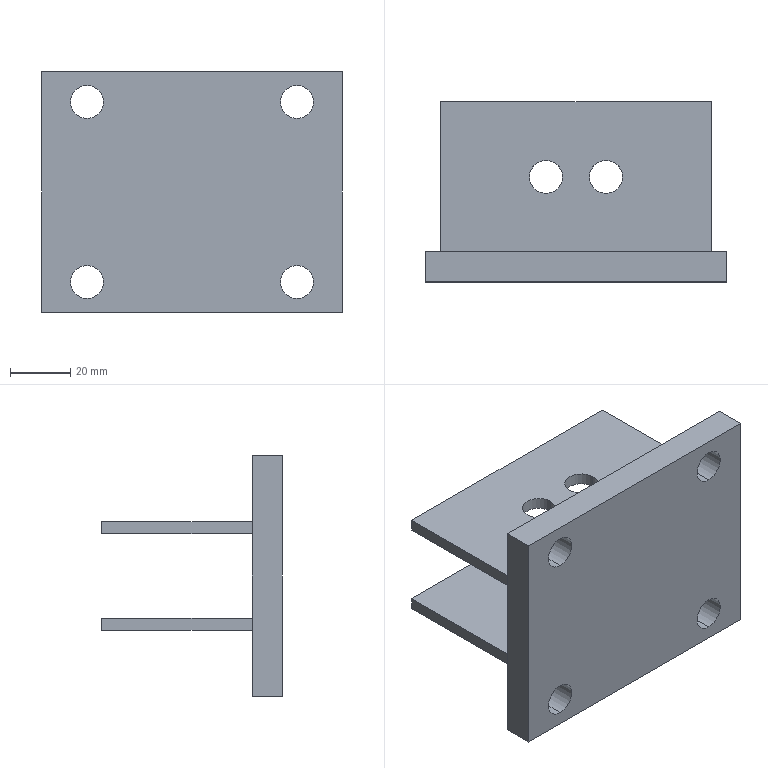Part | SolidWorks | features ICE 3, Extrusion 1, MirrorPattern 1 | 1 solid | 32 faces | box 100 x 60 x 80 mm | volume 110678 mm3 | cylinder 16 | plane 16 | commonest cylinder face diameters 11 x16
STEP:
#1=CARTESIAN_POINT('',(4.5,0.,-32.));
#2=VERTEX_POINT('',#1);
#3=CARTESIAN_POINT('',(15.5,0.,-32.));
#4=VERTEX_POINT('',#3);
#5=CARTESIAN_POINT('',(10.,0.,-32.));
#6=DIRECTION('',(0.,0.,1.));
#7=DIRECTION('',(1.,0.,0.));
#8=AXIS2_PLACEMENT_3D('',#5,#6,#7);
#9=CIRCLE('',#8,5.5);
#10=EDGE_CURVE('',#2,#4,#9,.T.);
#11=ORIENTED_EDGE('',*,*,#10,.F.);
#12=CARTESIAN_POINT('',(4.5,0.,-28.));
#13=VERTEX_POINT('',#12);
#14=CARTESIAN_POINT('',(4.5,0.,-54.));
#15=DIRECTION('',(0.,0.,1.));
#16=VECTOR('',#15,1000.);
#17=LINE('',#14,#16);
#18=EDGE_CURVE('',#2,#13,#17,.T.);
#19=ORIENTED_EDGE('',*,*,#18,.T.);
#20=CARTESIAN_POINT('',(15.5,0.,-28.));
#21=VERTEX_POINT('',#20);
#22=CARTESIAN_POINT('',(10.,0.,-28.));
#23=DIRECTION('',(0.,0.,1.));
#24=DIRECTION('',(1.,0.,0.));
#25=AXIS2_PLACEMENT_3D('',#22,#23,#24);
#26=CIRCLE('',#25,5.5);
#27=EDGE_CURVE('',#13,#21,#26,.T.);
#28=ORIENTED_EDGE('',*,*,#27,.T.);
#29=CARTESIAN_POINT('',(15.5,0.,-54.));
#30=DIRECTION('',(0.,0.,1.));
#31=VECTOR('',#30,1000.);
#32=LINE('',#29,#31);
#33=EDGE_CURVE('',#4,#21,#32,.T.);
#34=ORIENTED_EDGE('',*,*,#33,.F.);
#35=EDGE_LOOP('',(#11,#19,#28,#34));
#36=FACE_OUTER_BOUND('',#35,.T.);
#37=CARTESIAN_POINT('',(10.,0.,-54.));
#38=DIRECTION('',(0.,0.,1.));
#39=DIRECTION('',(1.,0.,0.));
#40=AXIS2_PLACEMENT_3D('',#37,#38,#39);
#41=CYLINDRICAL_SURFACE('',#40,5.5);
#42=ADVANCED_FACE('',(#36),#41,.F.);
#43=CARTESIAN_POINT('',(-15.5,0.,-32.));
#44=VERTEX_POINT('',#43);
#45=CARTESIAN_POINT('',(-4.5,0.,-32.));
#46=VERTEX_POINT('',#45);
#47=CARTESIAN_POINT('',(-10.,0.,-32.));
#48=DIRECTION('',(0.,0.,1.));
#49=DIRECTION('',(1.,0.,0.));
#50=AXIS2_PLACEMENT_3D('',#47,#48,#49);
#51=CIRCLE('',#50,5.5);
#52=EDGE_CURVE('',#44,#46,#51,.T.);
#53=ORIENTED_EDGE('',*,*,#52,.F.);
#54=CARTESIAN_POINT('',(-15.5,0.,-28.));
#55=VERTEX_POINT('',#54);
#56=CARTESIAN_POINT('',(-15.5,0.,-54.));
#57=DIRECTION('',(0.,0.,1.));
#58=VECTOR('',#57,1000.);
#59=LINE('',#56,#58);
#60=EDGE_CURVE('',#44,#55,#59,.T.);
#61=ORIENTED_EDGE('',*,*,#60,.T.);
#62=CARTESIAN_POINT('',(-4.5,0.,-28.));
#63=VERTEX_POINT('',#62);
#64=CARTESIAN_POINT('',(-10.,0.,-28.));
#65=DIRECTION('',(0.,0.,1.));
#66=DIRECTION('',(1.,0.,0.));
#67=AXIS2_PLACEMENT_3D('',#64,#65,#66);
#68=CIRCLE('',#67,5.5);
#69=EDGE_CURVE('',#55,#63,#68,.T.);
#70=ORIENTED_EDGE('',*,*,#69,.T.);
#71=CARTESIAN_POINT('',(-4.5,0.,-54.));
#72=DIRECTION('',(0.,0.,1.));
#73=VECTOR('',#72,1000.);
#74=LINE('',#71,#73);
#75=EDGE_CURVE('',#46,#63,#74,.T.);
#76=ORIENTED_EDGE('',*,*,#75,.F.);
#77=EDGE_LOOP('',(#53,#61,#70,#76));
#78=FACE_OUTER_BOUND('',#77,.T.);
#79=CARTESIAN_POINT('',(-10.,0.,-54.));
#80=DIRECTION('',(0.,0.,1.));
#81=DIRECTION('',(1.,0.,0.));
#82=AXIS2_PLACEMENT_3D('',#79,#80,#81);
#83=CYLINDRICAL_SURFACE('',#82,5.5);
#84=ADVANCED_FACE('',(#78),#83,.F.);
#85=CARTESIAN_POINT('',(-35.,-35.,-38.5));
#86=VERTEX_POINT('',#85);
#87=CARTESIAN_POINT('',(-35.,-35.,-49.5));
#88=VERTEX_POINT('',#87);
#89=CARTESIAN_POINT('',(-35.,-35.,-44.));
#90=DIRECTION('',(0.,-1.,0.));
#91=DIRECTION('',(0.,0.,-1.));
#92=AXIS2_PLACEMENT_3D('',#89,#90,#91);
#93=CIRCLE('',#92,5.5);
#94=EDGE_CURVE('',#86,#88,#93,.T.);
#95=ORIENTED_EDGE('',*,*,#94,.T.);
#96=CARTESIAN_POINT('',(-35.,-25.,-49.5));
#97=VERTEX_POINT('',#96);
#98=CARTESIAN_POINT('',(-35.,-35.,-49.5));
#99=DIRECTION('',(0.,1.,0.));
#100=VECTOR('',#99,1000.);
#101=LINE('',#98,#100);
#102=EDGE_CURVE('',#88,#97,#101,.T.);
#103=ORIENTED_EDGE('',*,*,#102,.T.);
#104=CARTESIAN_POINT('',(-35.,-25.,-38.5));
#105=VERTEX_POINT('',#104);
#106=CARTESIAN_POINT('',(-35.,-25.,-44.));
#107=DIRECTION('',(0.,-1.,0.));
#108=DIRECTION('',(0.,0.,-1.));
#109=AXIS2_PLACEMENT_3D('',#106,#107,#108);
#110=CIRCLE('',#109,5.5);
#111=EDGE_CURVE('',#105,#97,#110,.T.);
#112=ORIENTED_EDGE('',*,*,#111,.F.);
#113=CARTESIAN_POINT('',(-35.,-35.,-38.5));
#114=DIRECTION('',(0.,1.,0.));
#115=VECTOR('',#114,1000.);
#116=LINE('',#113,#115);
#117=EDGE_CURVE('',#86,#105,#116,.T.);
#118=ORIENTED_EDGE('',*,*,#117,.F.);
#119=EDGE_LOOP('',(#95,#103,#112,#118));
#120=FACE_OUTER_BOUND('',#119,.T.);
#121=CARTESIAN_POINT('',(-35.,-35.,-44.));
#122=DIRECTION('',(0.,1.,0.));
#123=DIRECTION('',(0.,0.,1.));
#124=AXIS2_PLACEMENT_3D('',#121,#122,#123);
#125=CYLINDRICAL_SURFACE('',#124,5.5);
#126=ADVANCED_FACE('',(#120),#125,.F.);
#127=CARTESIAN_POINT('',(35.,-35.,-38.5));
#128=VERTEX_POINT('',#127);
#129=CARTESIAN_POINT('',(35.,-35.,-49.5));
#130=VERTEX_POINT('',#129);
#131=CARTESIAN_POINT('',(35.,-35.,-44.));
#132=DIRECTION('',(0.,-1.,0.));
#133=DIRECTION('',(0.,0.,-1.));
#134=AXIS2_PLACEMENT_3D('',#131,#132,#133);
#135=CIRCLE('',#134,5.5);
#136=EDGE_CURVE('',#128,#130,#135,.T.);
#137=ORIENTED_EDGE('',*,*,#136,.T.);
#138=CARTESIAN_POINT('',(35.,-25.,-49.5));
#139=VERTEX_POINT('',#138);
#140=CARTESIAN_POINT('',(35.,-35.,-49.5));
#141=DIRECTION('',(0.,1.,0.));
#142=VECTOR('',#141,1000.);
#143=LINE('',#140,#142);
#144=EDGE_CURVE('',#130,#139,#143,.T.);
#145=ORIENTED_EDGE('',*,*,#144,.T.);
#146=CARTESIAN_POINT('',(35.,-25.,-38.5));
#147=VERTEX_POINT('',#146);
#148=CARTESIAN_POINT('',(35.,-25.,-44.));
#149=DIRECTION('',(0.,-1.,0.));
#150=DIRECTION('',(0.,0.,-1.));
#151=AXIS2_PLACEMENT_3D('',#148,#149,#150);
#152=CIRCLE('',#151,5.5);
#153=EDGE_CURVE('',#147,#139,#152,.T.);
#154=ORIENTED_EDGE('',*,*,#153,.F.);
#155=CARTESIAN_POINT('',(35.,-35.,-38.5));
#156=DIRECTION('',(0.,1.,0.));
#157=VECTOR('',#156,1000.);
#158=LINE('',#155,#157);
#159=EDGE_CURVE('',#128,#147,#158,.T.);
#160=ORIENTED_EDGE('',*,*,#159,.F.);
#161=EDGE_LOOP('',(#137,#145,#154,#160));
#162=FACE_OUTER_BOUND('',#161,.T.);
#163=CARTESIAN_POINT('',(35.,-35.,-44.));
#164=DIRECTION('',(0.,1.,0.));
#165=DIRECTION('',(0.,0.,1.));
#166=AXIS2_PLACEMENT_3D('',#163,#164,#165);
#167=CYLINDRICAL_SURFACE('',#166,5.5);
#168=ADVANCED_FACE('',(#162),#167,.F.);
#169=CARTESIAN_POINT('',(35.,-35.,21.5));
#170=VERTEX_POINT('',#169);
#171=CARTESIAN_POINT('',(35.,-35.,10.5));
#172=VERTEX_POINT('',#171);
#173=CARTESIAN_POINT('',(35.,-35.,16.));
#174=DIRECTION('',(0.,-1.,0.));
#175=DIRECTION('',(0.,0.,-1.));
#176=AXIS2_PLACEMENT_3D('',#173,#174,#175);
#177=CIRCLE('',#176,5.5);
#178=EDGE_CURVE('',#170,#172,#177,.T.);
#179=ORIENTED_EDGE('',*,*,#178,.T.);
#180=CARTESIAN_POINT('',(35.,-25.,10.5));
#181=VERTEX_POINT('',#180);
#182=CARTESIAN_POINT('',(35.,-35.,10.5));
#183=DIRECTION('',(0.,1.,0.));
#184=VECTOR('',#183,1000.);
#185=LINE('',#182,#184);
#186=EDGE_CURVE('',#172,#181,#185,.T.);
#187=ORIENTED_EDGE('',*,*,#186,.T.);
#188=CARTESIAN_POINT('',(35.,-25.,21.5));
#189=VERTEX_POINT('',#188);
#190=CARTESIAN_POINT('',(35.,-25.,16.));
#191=DIRECTION('',(0.,-1.,0.));
#192=DIRECTION('',(0.,0.,-1.));
#193=AXIS2_PLACEMENT_3D('',#190,#191,#192);
#194=CIRCLE('',#193,5.5);
#195=EDGE_CURVE('',#189,#181,#194,.T.);
#196=ORIENTED_EDGE('',*,*,#195,.F.);
#197=CARTESIAN_POINT('',(35.,-35.,21.5));
#198=DIRECTION('',(0.,1.,0.));
#199=VECTOR('',#198,1000.);
#200=LINE('',#197,#199);
#201=EDGE_CURVE('',#170,#189,#200,.T.);
#202=ORIENTED_EDGE('',*,*,#201,.F.);
#203=EDGE_LOOP('',(#179,#187,#196,#202));
#204=FACE_OUTER_BOUND('',#203,.T.);
#205=CARTESIAN_POINT('',(35.,-35.,16.));
#206=DIRECTION('',(0.,1.,0.));
#207=DIRECTION('',(0.,0.,1.));
#208=AXIS2_PLACEMENT_3D('',#205,#206,#207);
#209=CYLINDRICAL_SURFACE('',#208,5.5);
#210=ADVANCED_FACE('',(#204),#209,.F.);
#211=CARTESIAN_POINT('',(-35.,-35.,21.5));
#212=VERTEX_POINT('',#211);
#213=CARTESIAN_POINT('',(-35.,-35.,10.5));
#214=VERTEX_POINT('',#213);
#215=CARTESIAN_POINT('',(-35.,-35.,16.));
#216=DIRECTION('',(0.,-1.,0.));
#217=DIRECTION('',(0.,0.,-1.));
#218=AXIS2_PLACEMENT_3D('',#215,#216,#217);
#219=CIRCLE('',#218,5.5);
#220=EDGE_CURVE('',#212,#214,#219,.T.);
#221=ORIENTED_EDGE('',*,*,#220,.T.);
#222=CARTESIAN_POINT('',(-35.,-25.,10.5));
#223=VERTEX_POINT('',#222);
#224=CARTESIAN_POINT('',(-35.,-35.,10.5));
#225=DIRECTION('',(0.,1.,0.));
#226=VECTOR('',#225,1000.);
#227=LINE('',#224,#226);
#228=EDGE_CURVE('',#214,#223,#227,.T.);
#229=ORIENTED_EDGE('',*,*,#228,.T.);
#230=CARTESIAN_POINT('',(-35.,-25.,21.5));
#231=VERTEX_POINT('',#230);
#232=CARTESIAN_POINT('',(-35.,-25.,16.));
#233=DIRECTION('',(0.,-1.,0.));
#234=DIRECTION('',(0.,0.,-1.));
#235=AXIS2_PLACEMENT_3D('',#232,#233,#234);
#236=CIRCLE('',#235,5.5);
#237=EDGE_CURVE('',#231,#223,#236,.T.);
#238=ORIENTED_EDGE('',*,*,#237,.F.);
#239=CARTESIAN_POINT('',(-35.,-35.,21.5));
#240=DIRECTION('',(0.,1.,0.));
#241=VECTOR('',#240,1000.);
#242=LINE('',#239,#241);
#243=EDGE_CURVE('',#212,#231,#242,.T.);
#244=ORIENTED_EDGE('',*,*,#243,.F.);
#245=EDGE_LOOP('',(#221,#229,#238,#244));
#246=FACE_OUTER_BOUND('',#245,.T.);
#247=CARTESIAN_POINT('',(-35.,-35.,16.));
#248=DIRECTION('',(0.,1.,0.));
#249=DIRECTION('',(0.,0.,1.));
#250=AXIS2_PLACEMENT_3D('',#247,#248,#249);
#251=CYLINDRICAL_SURFACE('',#250,5.5);
#252=ADVANCED_FACE('',(#246),#251,.F.);
#253=CARTESIAN_POINT('',(4.5,0.,0.));
#254=VERTEX_POINT('',#253);
#255=CARTESIAN_POINT('',(15.5,0.,0.));
#256=VERTEX_POINT('',#255);
#257=CARTESIAN_POINT('',(10.,0.,0.));
#258=DIRECTION('',(0.,0.,1.));
#259=DIRECTION('',(1.,0.,0.));
#260=AXIS2_PLACEMENT_3D('',#257,#258,#259);
#261=CIRCLE('',#260,5.5);
#262=EDGE_CURVE('',#254,#256,#261,.T.);
#263=ORIENTED_EDGE('',*,*,#262,.F.);
#264=CARTESIAN_POINT('',(4.5,0.,4.));
#265=VERTEX_POINT('',#264);
#266=CARTESIAN_POINT('',(4.5,0.,0.));
#267=DIRECTION('',(0.,0.,1.));
#268=VECTOR('',#267,1000.);
#269=LINE('',#266,#268);
#270=EDGE_CURVE('',#254,#265,#269,.T.);
#271=ORIENTED_EDGE('',*,*,#270,.T.);
#272=CARTESIAN_POINT('',(15.5,0.,4.));
#273=VERTEX_POINT('',#272);
#274=CARTESIAN_POINT('',(10.,0.,4.));
#275=DIRECTION('',(0.,0.,1.));
#276=DIRECTION('',(1.,0.,0.));
#277=AXIS2_PLACEMENT_3D('',#274,#275,#276);
#278=CIRCLE('',#277,5.5);
#279=EDGE_CURVE('',#265,#273,#278,.T.);
#280=ORIENTED_EDGE('',*,*,#279,.T.);
#281=CARTESIAN_POINT('',(15.5,0.,0.));
#282=DIRECTION('',(0.,0.,1.));
#283=VECTOR('',#282,1000.);
#284=LINE('',#281,#283);
#285=EDGE_CURVE('',#256,#273,#284,.T.);
#286=ORIENTED_EDGE('',*,*,#285,.F.);
#287=EDGE_LOOP('',(#263,#271,#280,#286));
#288=FACE_OUTER_BOUND('',#287,.T.);
#289=CARTESIAN_POINT('',(10.,0.,0.));
#290=DIRECTION('',(0.,0.,1.));
#291=DIRECTION('',(1.,0.,0.));
#292=AXIS2_PLACEMENT_3D('',#289,#290,#291);
#293=CYLINDRICAL_SURFACE('',#292,5.5);
#294=ADVANCED_FACE('',(#288),#293,.F.);
#295=CARTESIAN_POINT('',(-15.5,0.,0.));
#296=VERTEX_POINT('',#295);
#297=CARTESIAN_POINT('',(-4.5,0.,0.));
#298=VERTEX_POINT('',#297);
#299=CARTESIAN_POINT('',(-10.,0.,0.));
#300=DIRECTION('',(0.,0.,1.));
#301=DIRECTION('',(1.,0.,0.));
#302=AXIS2_PLACEMENT_3D('',#299,#300,#301);
#303=CIRCLE('',#302,5.5);
#304=EDGE_CURVE('',#296,#298,#303,.T.);
#305=ORIENTED_EDGE('',*,*,#304,.F.);
#306=CARTESIAN_POINT('',(-15.5,0.,4.));
#307=VERTEX_POINT('',#306);
#308=CARTESIAN_POINT('',(-15.5,0.,0.));
#309=DIRECTION('',(0.,0.,1.));
#310=VECTOR('',#309,1000.);
#311=LINE('',#308,#310);
#312=EDGE_CURVE('',#296,#307,#311,.T.);
#313=ORIENTED_EDGE('',*,*,#312,.T.);
#314=CARTESIAN_POINT('',(-4.5,0.,4.));
#315=VERTEX_POINT('',#314);
#316=CARTESIAN_POINT('',(-10.,0.,4.));
#317=DIRECTION('',(0.,0.,1.));
#318=DIRECTION('',(1.,0.,0.));
#319=AXIS2_PLACEMENT_3D('',#316,#317,#318);
#320=CIRCLE('',#319,5.5);
#321=EDGE_CURVE('',#307,#315,#320,.T.);
#322=ORIENTED_EDGE('',*,*,#321,.T.);
#323=CARTESIAN_POINT('',(-4.5,0.,0.));
#324=DIRECTION('',(0.,0.,1.));
#325=VECTOR('',#324,1000.);
#326=LINE('',#323,#325);
#327=EDGE_CURVE('',#298,#315,#326,.T.);
#328=ORIENTED_EDGE('',*,*,#327,.F.);
#329=EDGE_LOOP('',(#305,#313,#322,#328));
#330=FACE_OUTER_BOUND('',#329,.T.);
#331=CARTESIAN_POINT('',(-10.,0.,0.));
#332=DIRECTION('',(0.,0.,1.));
#333=DIRECTION('',(1.,0.,0.));
#334=AXIS2_PLACEMENT_3D('',#331,#332,#333);
#335=CYLINDRICAL_SURFACE('',#334,5.5);
#336=ADVANCED_FACE('',(#330),#335,.F.);
#337=CARTESIAN_POINT('',(-45.,-25.,4.));
#338=VERTEX_POINT('',#337);
#339=CARTESIAN_POINT('',(45.,-25.,4.));
#340=VERTEX_POINT('',#339);
#341=CARTESIAN_POINT('',(-45.,-25.,4.));
#342=DIRECTION('',(1.,0.,0.));
#343=VECTOR('',#342,1000.);
#344=LINE('',#341,#343);
#345=EDGE_CURVE('',#338,#340,#344,.T.);
#346=ORIENTED_EDGE('',*,*,#345,.F.);
#347=CARTESIAN_POINT('',(-45.,-25.,0.));
#348=VERTEX_POINT('',#347);
#349=CARTESIAN_POINT('',(-45.,-25.,4.));
#350=DIRECTION('',(0.,0.,-1.));
#351=VECTOR('',#350,1000.);
#352=LINE('',#349,#351);
#353=EDGE_CURVE('',#338,#348,#352,.T.);
#354=ORIENTED_EDGE('',*,*,#353,.T.);
#355=CARTESIAN_POINT('',(45.,-25.,0.));
#356=VERTEX_POINT('',#355);
#357=CARTESIAN_POINT('',(-45.,-25.,0.));
#358=DIRECTION('',(1.,0.,0.));
#359=VECTOR('',#358,1000.);
#360=LINE('',#357,#359);
#361=EDGE_CURVE('',#348,#356,#360,.T.);
#362=ORIENTED_EDGE('',*,*,#361,.T.);
#363=CARTESIAN_POINT('',(45.,-25.,4.));
#364=DIRECTION('',(0.,0.,-1.));
#365=VECTOR('',#364,1000.);
#366=LINE('',#363,#365);
#367=EDGE_CURVE('',#340,#356,#366,.T.);
#368=ORIENTED_EDGE('',*,*,#367,.F.);
#369=EDGE_LOOP('',(#346,#354,#362,#368));
#370=FACE_BOUND('',#369,.T.);
#371=ORIENTED_EDGE('',*,*,#153,.T.);
#372=CARTESIAN_POINT('',(35.,-25.,-44.));
#373=DIRECTION('',(0.,-1.,0.));
#374=DIRECTION('',(0.,0.,-1.));
#375=AXIS2_PLACEMENT_3D('',#372,#373,#374);
#376=CIRCLE('',#375,5.5);
#377=EDGE_CURVE('',#139,#147,#376,.T.);
#378=ORIENTED_EDGE('',*,*,#377,.T.);
#379=EDGE_LOOP('',(#371,#378));
#380=FACE_BOUND('',#379,.T.);
#381=ORIENTED_EDGE('',*,*,#237,.T.);
#382=CARTESIAN_POINT('',(-35.,-25.,16.));
#383=DIRECTION('',(0.,-1.,0.));
#384=DIRECTION('',(0.,0.,-1.));
#385=AXIS2_PLACEMENT_3D('',#382,#383,#384);
#386=CIRCLE('',#385,5.5);
#387=EDGE_CURVE('',#223,#231,#386,.T.);
#388=ORIENTED_EDGE('',*,*,#387,.T.);
#389=EDGE_LOOP('',(#381,#388));
#390=FACE_BOUND('',#389,.T.);
#391=CARTESIAN_POINT('',(50.,-25.,-54.));
#392=VERTEX_POINT('',#391);
#393=CARTESIAN_POINT('',(50.,-25.,26.));
#394=VERTEX_POINT('',#393);
#395=CARTESIAN_POINT('',(50.,-25.,-54.));
#396=DIRECTION('',(0.,0.,1.));
#397=VECTOR('',#396,1000.);
#398=LINE('',#395,#397);
#399=EDGE_CURVE('',#392,#394,#398,.T.);
#400=ORIENTED_EDGE('',*,*,#399,.F.);
#401=CARTESIAN_POINT('',(-50.,-25.,-54.));
#402=VERTEX_POINT('',#401);
#403=CARTESIAN_POINT('',(-50.,-25.,-54.));
#404=DIRECTION('',(1.,0.,0.));
#405=VECTOR('',#404,1000.);
#406=LINE('',#403,#405);
#407=EDGE_CURVE('',#402,#392,#406,.T.);
#408=ORIENTED_EDGE('',*,*,#407,.F.);
#409=CARTESIAN_POINT('',(-50.,-25.,26.));
#410=VERTEX_POINT('',#409);
#411=CARTESIAN_POINT('',(-50.,-25.,-54.));
#412=DIRECTION('',(0.,0.,-1.));
#413=VECTOR('',#412,1000.);
#414=LINE('',#411,#413);
#415=EDGE_CURVE('',#410,#402,#414,.T.);
#416=ORIENTED_EDGE('',*,*,#415,.F.);
#417=CARTESIAN_POINT('',(-50.,-25.,26.));
#418=DIRECTION('',(-1.,0.,0.));
#419=VECTOR('',#418,1000.);
#420=LINE('',#417,#419);
#421=EDGE_CURVE('',#394,#410,#420,.T.);
#422=ORIENTED_EDGE('',*,*,#421,.F.);
#423=EDGE_LOOP('',(#400,#408,#416,#422));
#424=FACE_OUTER_BOUND('',#423,.T.);
#425=ORIENTED_EDGE('',*,*,#195,.T.);
#426=CARTESIAN_POINT('',(35.,-25.,16.));
#427=DIRECTION('',(0.,-1.,0.));
#428=DIRECTION('',(0.,0.,-1.));
#429=AXIS2_PLACEMENT_3D('',#426,#427,#428);
#430=CIRCLE('',#429,5.5);
#431=EDGE_CURVE('',#181,#189,#430,.T.);
#432=ORIENTED_EDGE('',*,*,#431,.T.);
#433=EDGE_LOOP('',(#425,#432));
#434=FACE_BOUND('',#433,.T.);
#435=ORIENTED_EDGE('',*,*,#111,.T.);
#436=CARTESIAN_POINT('',(-35.,-25.,-44.));
#437=DIRECTION('',(0.,-1.,0.));
#438=DIRECTION('',(0.,0.,-1.));
#439=AXIS2_PLACEMENT_3D('',#436,#437,#438);
#440=CIRCLE('',#439,5.5);
#441=EDGE_CURVE('',#97,#105,#440,.T.);
#442=ORIENTED_EDGE('',*,*,#441,.T.);
#443=EDGE_LOOP('',(#435,#442));
#444=FACE_BOUND('',#443,.T.);
#445=CARTESIAN_POINT('',(-45.,-25.,-32.));
#446=VERTEX_POINT('',#445);
#447=CARTESIAN_POINT('',(-45.,-25.,-28.));
#448=VERTEX_POINT('',#447);
#449=CARTESIAN_POINT('',(-45.,-25.,-32.));
#450=DIRECTION('',(0.,0.,1.));
#451=VECTOR('',#450,1000.);
#452=LINE('',#449,#451);
#453=EDGE_CURVE('',#446,#448,#452,.T.);
#454=ORIENTED_EDGE('',*,*,#453,.F.);
#455=CARTESIAN_POINT('',(45.,-25.,-32.));
#456=VERTEX_POINT('',#455);
#457=CARTESIAN_POINT('',(-45.,-25.,-32.));
#458=DIRECTION('',(1.,0.,0.));
#459=VECTOR('',#458,1000.);
#460=LINE('',#457,#459);
#461=EDGE_CURVE('',#446,#456,#460,.T.);
#462=ORIENTED_EDGE('',*,*,#461,.T.);
#463=CARTESIAN_POINT('',(45.,-25.,-28.));
#464=VERTEX_POINT('',#463);
#465=CARTESIAN_POINT('',(45.,-25.,-32.));
#466=DIRECTION('',(0.,0.,1.));
#467=VECTOR('',#466,1000.);
#468=LINE('',#465,#467);
#469=EDGE_CURVE('',#456,#464,#468,.T.);
#470=ORIENTED_EDGE('',*,*,#469,.T.);
#471=CARTESIAN_POINT('',(-45.,-25.,-28.));
#472=DIRECTION('',(1.,0.,0.));
#473=VECTOR('',#472,1000.);
#474=LINE('',#471,#473);
#475=EDGE_CURVE('',#448,#464,#474,.T.);
#476=ORIENTED_EDGE('',*,*,#475,.F.);
#477=EDGE_LOOP('',(#454,#462,#470,#476));
#478=FACE_BOUND('',#477,.T.);
#479=CARTESIAN_POINT('',(0.,-25.,0.));
#480=DIRECTION('',(0.,1.,0.));
#481=DIRECTION('',(0.,0.,1.));
#482=AXIS2_PLACEMENT_3D('',#479,#480,#481);
#483=PLANE('',#482);
#484=ADVANCED_FACE('',(#370,#380,#390,#424,#434,#444,#478),#483,.T.);
#485=CARTESIAN_POINT('',(45.,25.,0.));
#486=VERTEX_POINT('',#485);
#487=CARTESIAN_POINT('',(45.,-25.,0.));
#488=DIRECTION('',(0.,1.,0.));
#489=VECTOR('',#488,1000.);
#490=LINE('',#487,#489);
#491=EDGE_CURVE('',#356,#486,#490,.T.);
#492=ORIENTED_EDGE('',*,*,#491,.T.);
#493=CARTESIAN_POINT('',(45.,25.,4.));
#494=VERTEX_POINT('',#493);
#495=CARTESIAN_POINT('',(45.,25.,4.));
#496=DIRECTION('',(0.,0.,-1.));
#497=VECTOR('',#496,1000.);
#498=LINE('',#495,#497);
#499=EDGE_CURVE('',#494,#486,#498,.T.);
#500=ORIENTED_EDGE('',*,*,#499,.F.);
#501=CARTESIAN_POINT('',(45.,-25.,4.));
#502=DIRECTION('',(0.,1.,0.));
#503=VECTOR('',#502,1000.);
#504=LINE('',#501,#503);
#505=EDGE_CURVE('',#340,#494,#504,.T.);
#506=ORIENTED_EDGE('',*,*,#505,.F.);
#507=ORIENTED_EDGE('',*,*,#367,.T.);
#508=EDGE_LOOP('',(#492,#500,#506,#507));
#509=FACE_OUTER_BOUND('',#508,.T.);
#510=CARTESIAN_POINT('',(45.,-25.,4.));
#511=DIRECTION('',(-1.,0.,0.));
#512=DIRECTION('',(0.,0.,1.));
#513=AXIS2_PLACEMENT_3D('',#510,#511,#512);
#514=PLANE('',#513);
#515=ADVANCED_FACE('',(#509),#514,.F.);
#516=CARTESIAN_POINT('',(-45.,25.,0.));
#517=VERTEX_POINT('',#516);
#518=CARTESIAN_POINT('',(-45.,25.,0.));
#519=DIRECTION('',(-1.,0.,0.));
#520=VECTOR('',#519,1000.);
#521=LINE('',#518,#520);
#522=EDGE_CURVE('',#486,#517,#521,.T.);
#523=ORIENTED_EDGE('',*,*,#522,.T.);
#524=CARTESIAN_POINT('',(-45.,25.,4.));
#525=VERTEX_POINT('',#524);
#526=CARTESIAN_POINT('',(-45.,25.,4.));
#527=DIRECTION('',(0.,0.,-1.));
#528=VECTOR('',#527,1000.);
#529=LINE('',#526,#528);
#530=EDGE_CURVE('',#525,#517,#529,.T.);
#531=ORIENTED_EDGE('',*,*,#530,.F.);
#532=CARTESIAN_POINT('',(-45.,25.,4.));
#533=DIRECTION('',(-1.,0.,0.));
#534=VECTOR('',#533,1000.);
#535=LINE('',#532,#534);
#536=EDGE_CURVE('',#494,#525,#535,.T.);
#537=ORIENTED_EDGE('',*,*,#536,.F.);
#538=ORIENTED_EDGE('',*,*,#499,.T.);
#539=EDGE_LOOP('',(#523,#531,#537,#538));
#540=FACE_OUTER_BOUND('',#539,.T.);
#541=CARTESIAN_POINT('',(-45.,25.,4.));
#542=DIRECTION('',(0.,-1.,0.));
#543=DIRECTION('',(0.,0.,-1.));
#544=AXIS2_PLACEMENT_3D('',#541,#542,#543);
#545=PLANE('',#544);
#546=ADVANCED_FACE('',(#540),#545,.F.);
#547=CARTESIAN_POINT('',(-45.,-25.,0.));
#548=DIRECTION('',(0.,-1.,0.));
#549=VECTOR('',#548,1000.);
#550=LINE('',#547,#549);
#551=EDGE_CURVE('',#517,#348,#550,.T.);
#552=ORIENTED_EDGE('',*,*,#551,.T.);
#553=ORIENTED_EDGE('',*,*,#353,.F.);
#554=CARTESIAN_POINT('',(-45.,-25.,4.));
#555=DIRECTION('',(0.,-1.,0.));
#556=VECTOR('',#555,1000.);
#557=LINE('',#554,#556);
#558=EDGE_CURVE('',#525,#338,#557,.T.);
#559=ORIENTED_EDGE('',*,*,#558,.F.);
#560=ORIENTED_EDGE('',*,*,#530,.T.);
#561=EDGE_LOOP('',(#552,#553,#559,#560));
#562=FACE_OUTER_BOUND('',#561,.T.);
#563=CARTESIAN_POINT('',(-45.,-25.,4.));
#564=DIRECTION('',(1.,0.,0.));
#565=DIRECTION('',(0.,0.,-1.));
#566=AXIS2_PLACEMENT_3D('',#563,#564,#565);
#567=PLANE('',#566);
#568=ADVANCED_FACE('',(#562),#567,.F.);
#569=CARTESIAN_POINT('',(10.,0.,4.));
#570=DIRECTION('',(0.,0.,1.));
#571=DIRECTION('',(1.,0.,0.));
#572=AXIS2_PLACEMENT_3D('',#569,#570,#571);
#573=CIRCLE('',#572,5.5);
#574=EDGE_CURVE('',#273,#265,#573,.T.);
#575=ORIENTED_EDGE('',*,*,#574,.F.);
#576=ORIENTED_EDGE('',*,*,#279,.F.);
#577=EDGE_LOOP('',(#575,#576));
#578=FACE_BOUND('',#577,.T.);
#579=CARTESIAN_POINT('',(-10.,0.,4.));
#580=DIRECTION('',(0.,0.,1.));
#581=DIRECTION('',(1.,0.,0.));
#582=AXIS2_PLACEMENT_3D('',#579,#580,#581);
#583=CIRCLE('',#582,5.5);
#584=EDGE_CURVE('',#315,#307,#583,.T.);
#585=ORIENTED_EDGE('',*,*,#584,.F.);
#586=ORIENTED_EDGE('',*,*,#321,.F.);
#587=EDGE_LOOP('',(#585,#586));
#588=FACE_BOUND('',#587,.T.);
#589=ORIENTED_EDGE('',*,*,#505,.T.);
#590=ORIENTED_EDGE('',*,*,#536,.T.);
#591=ORIENTED_EDGE('',*,*,#558,.T.);
#592=ORIENTED_EDGE('',*,*,#345,.T.);
#593=EDGE_LOOP('',(#589,#590,#591,#592));
#594=FACE_OUTER_BOUND('',#593,.T.);
#595=CARTESIAN_POINT('',(0.,0.,4.));
#596=DIRECTION('',(0.,0.,-1.));
#597=DIRECTION('',(-1.,0.,0.));
#598=AXIS2_PLACEMENT_3D('',#595,#596,#597);
#599=PLANE('',#598);
#600=ADVANCED_FACE('',(#578,#588,#594),#599,.F.);
#601=CARTESIAN_POINT('',(10.,0.,0.));
#602=DIRECTION('',(0.,0.,1.));
#603=DIRECTION('',(1.,0.,0.));
#604=AXIS2_PLACEMENT_3D('',#601,#602,#603);
#605=CIRCLE('',#604,5.5);
#606=EDGE_CURVE('',#256,#254,#605,.T.);
#607=ORIENTED_EDGE('',*,*,#606,.T.);
#608=ORIENTED_EDGE('',*,*,#262,.T.);
#609=EDGE_LOOP('',(#607,#608));
#610=FACE_BOUND('',#609,.T.);
#611=CARTESIAN_POINT('',(-10.,0.,0.));
#612=DIRECTION('',(0.,0.,1.));
#613=DIRECTION('',(1.,0.,0.));
#614=AXIS2_PLACEMENT_3D('',#611,#612,#613);
#615=CIRCLE('',#614,5.5);
#616=EDGE_CURVE('',#298,#296,#615,.T.);
#617=ORIENTED_EDGE('',*,*,#616,.T.);
#618=ORIENTED_EDGE('',*,*,#304,.T.);
#619=EDGE_LOOP('',(#617,#618));
#620=FACE_BOUND('',#619,.T.);
#621=ORIENTED_EDGE('',*,*,#491,.F.);
#622=ORIENTED_EDGE('',*,*,#361,.F.);
#623=ORIENTED_EDGE('',*,*,#551,.F.);
#624=ORIENTED_EDGE('',*,*,#522,.F.);
#625=EDGE_LOOP('',(#621,#622,#623,#624));
#626=FACE_OUTER_BOUND('',#625,.T.);
#627=CARTESIAN_POINT('',(0.,0.,0.));
#628=DIRECTION('',(0.,0.,-1.));
#629=DIRECTION('',(-1.,0.,0.));
#630=AXIS2_PLACEMENT_3D('',#627,#628,#629);
#631=PLANE('',#630);
#632=ADVANCED_FACE('',(#610,#620,#626),#631,.T.);
#633=ORIENTED_EDGE('',*,*,#312,.F.);
#634=ORIENTED_EDGE('',*,*,#616,.F.);
#635=ORIENTED_EDGE('',*,*,#327,.T.);
#636=ORIENTED_EDGE('',*,*,#584,.T.);
#637=EDGE_LOOP('',(#633,#634,#635,#636));
#638=FACE_OUTER_BOUND('',#637,.T.);
#639=CARTESIAN_POINT('',(-10.,0.,0.));
#640=DIRECTION('',(0.,0.,1.));
#641=DIRECTION('',(1.,0.,0.));
#642=AXIS2_PLACEMENT_3D('',#639,#640,#641);
#643=CYLINDRICAL_SURFACE('',#642,5.5);
#644=ADVANCED_FACE('',(#638),#643,.F.);
#645=ORIENTED_EDGE('',*,*,#270,.F.);
#646=ORIENTED_EDGE('',*,*,#606,.F.);
#647=ORIENTED_EDGE('',*,*,#285,.T.);
#648=ORIENTED_EDGE('',*,*,#574,.T.);
#649=EDGE_LOOP('',(#645,#646,#647,#648));
#650=FACE_OUTER_BOUND('',#649,.T.);
#651=CARTESIAN_POINT('',(10.,0.,0.));
#652=DIRECTION('',(0.,0.,1.));
#653=DIRECTION('',(1.,0.,0.));
#654=AXIS2_PLACEMENT_3D('',#651,#652,#653);
#655=CYLINDRICAL_SURFACE('',#654,5.5);
#656=ADVANCED_FACE('',(#650),#655,.F.);
#657=ORIENTED_EDGE('',*,*,#136,.F.);
#658=CARTESIAN_POINT('',(35.,-35.,-44.));
#659=DIRECTION('',(0.,-1.,0.));
#660=DIRECTION('',(0.,0.,-1.));
#661=AXIS2_PLACEMENT_3D('',#658,#659,#660);
#662=CIRCLE('',#661,5.5);
#663=EDGE_CURVE('',#130,#128,#662,.T.);
#664=ORIENTED_EDGE('',*,*,#663,.F.);
#665=EDGE_LOOP('',(#657,#664));
#666=FACE_BOUND('',#665,.T.);
#667=ORIENTED_EDGE('',*,*,#220,.F.);
#668=CARTESIAN_POINT('',(-35.,-35.,16.));
#669=DIRECTION('',(0.,-1.,0.));
#670=DIRECTION('',(0.,0.,-1.));
#671=AXIS2_PLACEMENT_3D('',#668,#669,#670);
#672=CIRCLE('',#671,5.5);
#673=EDGE_CURVE('',#214,#212,#672,.T.);
#674=ORIENTED_EDGE('',*,*,#673,.F.);
#675=EDGE_LOOP('',(#667,#674));
#676=FACE_BOUND('',#675,.T.);
#677=CARTESIAN_POINT('',(50.,-35.,-54.));
#678=VERTEX_POINT('',#677);
#679=CARTESIAN_POINT('',(50.,-35.,26.));
#680=VERTEX_POINT('',#679);
#681=CARTESIAN_POINT('',(50.,-35.,-54.));
#682=DIRECTION('',(0.,0.,1.));
#683=VECTOR('',#682,1000.);
#684=LINE('',#681,#683);
#685=EDGE_CURVE('',#678,#680,#684,.T.);
#686=ORIENTED_EDGE('',*,*,#685,.T.);
#687=CARTESIAN_POINT('',(-50.,-35.,26.));
#688=VERTEX_POINT('',#687);
#689=CARTESIAN_POINT('',(-50.,-35.,26.));
#690=DIRECTION('',(-1.,0.,0.));
#691=VECTOR('',#690,1000.);
#692=LINE('',#689,#691);
#693=EDGE_CURVE('',#680,#688,#692,.T.);
#694=ORIENTED_EDGE('',*,*,#693,.T.);
#695=CARTESIAN_POINT('',(-50.,-35.,-54.));
#696=VERTEX_POINT('',#695);
#697=CARTESIAN_POINT('',(-50.,-35.,-54.));
#698=DIRECTION('',(0.,0.,-1.));
#699=VECTOR('',#698,1000.);
#700=LINE('',#697,#699);
#701=EDGE_CURVE('',#688,#696,#700,.T.);
#702=ORIENTED_EDGE('',*,*,#701,.T.);
#703=CARTESIAN_POINT('',(-50.,-35.,-54.));
#704=DIRECTION('',(1.,0.,0.));
#705=VECTOR('',#704,1000.);
#706=LINE('',#703,#705);
#707=EDGE_CURVE('',#696,#678,#706,.T.);
#708=ORIENTED_EDGE('',*,*,#707,.T.);
#709=EDGE_LOOP('',(#686,#694,#702,#708));
#710=FACE_OUTER_BOUND('',#709,.T.);
#711=ORIENTED_EDGE('',*,*,#178,.F.);
#712=CARTESIAN_POINT('',(35.,-35.,16.));
#713=DIRECTION('',(0.,-1.,0.));
#714=DIRECTION('',(0.,0.,-1.));
#715=AXIS2_PLACEMENT_3D('',#712,#713,#714);
#716=CIRCLE('',#715,5.5);
#717=EDGE_CURVE('',#172,#170,#716,.T.);
#718=ORIENTED_EDGE('',*,*,#717,.F.);
#719=EDGE_LOOP('',(#711,#718));
#720=FACE_BOUND('',#719,.T.);
#721=ORIENTED_EDGE('',*,*,#94,.F.);
#722=CARTESIAN_POINT('',(-35.,-35.,-44.));
#723=DIRECTION('',(0.,-1.,0.));
#724=DIRECTION('',(0.,0.,-1.));
#725=AXIS2_PLACEMENT_3D('',#722,#723,#724);
#726=CIRCLE('',#725,5.5);
#727=EDGE_CURVE('',#88,#86,#726,.T.);
#728=ORIENTED_EDGE('',*,*,#727,.F.);
#729=EDGE_LOOP('',(#721,#728));
#730=FACE_BOUND('',#729,.T.);
#731=CARTESIAN_POINT('',(0.,-35.,0.));
#732=DIRECTION('',(0.,1.,0.));
#733=DIRECTION('',(0.,0.,1.));
#734=AXIS2_PLACEMENT_3D('',#731,#732,#733);
#735=PLANE('',#734);
#736=ADVANCED_FACE('',(#666,#676,#710,#720,#730),#735,.F.);
#737=ORIENTED_EDGE('',*,*,#399,.T.);
#738=CARTESIAN_POINT('',(50.,-35.,26.));
#739=DIRECTION('',(0.,1.,0.));
#740=VECTOR('',#739,1000.);
#741=LINE('',#738,#740);
#742=EDGE_CURVE('',#680,#394,#741,.T.);
#743=ORIENTED_EDGE('',*,*,#742,.F.);
#744=ORIENTED_EDGE('',*,*,#685,.F.);
#745=CARTESIAN_POINT('',(50.,-35.,-54.));
#746=DIRECTION('',(0.,1.,0.));
#747=VECTOR('',#746,1000.);
#748=LINE('',#745,#747);
#749=EDGE_CURVE('',#678,#392,#748,.T.);
#750=ORIENTED_EDGE('',*,*,#749,.T.);
#751=EDGE_LOOP('',(#737,#743,#744,#750));
#752=FACE_OUTER_BOUND('',#751,.T.);
#753=CARTESIAN_POINT('',(50.,-35.,-54.));
#754=DIRECTION('',(-1.,0.,0.));
#755=DIRECTION('',(0.,0.,1.));
#756=AXIS2_PLACEMENT_3D('',#753,#754,#755);
#757=PLANE('',#756);
#758=ADVANCED_FACE('',(#752),#757,.F.);
#759=ORIENTED_EDGE('',*,*,#421,.T.);
#760=CARTESIAN_POINT('',(-50.,-35.,26.));
#761=DIRECTION('',(0.,1.,0.));
#762=VECTOR('',#761,1000.);
#763=LINE('',#760,#762);
#764=EDGE_CURVE('',#688,#410,#763,.T.);
#765=ORIENTED_EDGE('',*,*,#764,.F.);
#766=ORIENTED_EDGE('',*,*,#693,.F.);
#767=ORIENTED_EDGE('',*,*,#742,.T.);
#768=EDGE_LOOP('',(#759,#765,#766,#767));
#769=FACE_OUTER_BOUND('',#768,.T.);
#770=CARTESIAN_POINT('',(-50.,-35.,26.));
#771=DIRECTION('',(0.,0.,-1.));
#772=DIRECTION('',(-1.,0.,0.));
#773=AXIS2_PLACEMENT_3D('',#770,#771,#772);
#774=PLANE('',#773);
#775=ADVANCED_FACE('',(#769),#774,.F.);
#776=ORIENTED_EDGE('',*,*,#415,.T.);
#777=CARTESIAN_POINT('',(-50.,-35.,-54.));
#778=DIRECTION('',(0.,1.,0.));
#779=VECTOR('',#778,1000.);
#780=LINE('',#777,#779);
#781=EDGE_CURVE('',#696,#402,#780,.T.);
#782=ORIENTED_EDGE('',*,*,#781,.F.);
#783=ORIENTED_EDGE('',*,*,#701,.F.);
#784=ORIENTED_EDGE('',*,*,#764,.T.);
#785=EDGE_LOOP('',(#776,#782,#783,#784));
#786=FACE_OUTER_BOUND('',#785,.T.);
#787=CARTESIAN_POINT('',(-50.,-35.,-54.));
#788=DIRECTION('',(1.,0.,0.));
#789=DIRECTION('',(0.,0.,-1.));
#790=AXIS2_PLACEMENT_3D('',#787,#788,#789);
#791=PLANE('',#790);
#792=ADVANCED_FACE('',(#786),#791,.F.);
#793=ORIENTED_EDGE('',*,*,#407,.T.);
#794=ORIENTED_EDGE('',*,*,#749,.F.);
#795=ORIENTED_EDGE('',*,*,#707,.F.);
#796=ORIENTED_EDGE('',*,*,#781,.T.);
#797=EDGE_LOOP('',(#793,#794,#795,#796));
#798=FACE_OUTER_BOUND('',#797,.T.);
#799=CARTESIAN_POINT('',(-50.,-35.,-54.));
#800=DIRECTION('',(0.,0.,1.));
#801=DIRECTION('',(1.,0.,0.));
#802=AXIS2_PLACEMENT_3D('',#799,#800,#801);
#803=PLANE('',#802);
#804=ADVANCED_FACE('',(#798),#803,.F.);
#805=ORIENTED_EDGE('',*,*,#228,.F.);
#806=ORIENTED_EDGE('',*,*,#673,.T.);
#807=ORIENTED_EDGE('',*,*,#243,.T.);
#808=ORIENTED_EDGE('',*,*,#387,.F.);
#809=EDGE_LOOP('',(#805,#806,#807,#808));
#810=FACE_OUTER_BOUND('',#809,.T.);
#811=CARTESIAN_POINT('',(-35.,-35.,16.));
#812=DIRECTION('',(0.,1.,0.));
#813=DIRECTION('',(0.,0.,1.));
#814=AXIS2_PLACEMENT_3D('',#811,#812,#813);
#815=CYLINDRICAL_SURFACE('',#814,5.5);
#816=ADVANCED_FACE('',(#810),#815,.F.);
#817=ORIENTED_EDGE('',*,*,#186,.F.);
#818=ORIENTED_EDGE('',*,*,#717,.T.);
#819=ORIENTED_EDGE('',*,*,#201,.T.);
#820=ORIENTED_EDGE('',*,*,#431,.F.);
#821=EDGE_LOOP('',(#817,#818,#819,#820));
#822=FACE_OUTER_BOUND('',#821,.T.);
#823=CARTESIAN_POINT('',(35.,-35.,16.));
#824=DIRECTION('',(0.,1.,0.));
#825=DIRECTION('',(0.,0.,1.));
#826=AXIS2_PLACEMENT_3D('',#823,#824,#825);
#827=CYLINDRICAL_SURFACE('',#826,5.5);
#828=ADVANCED_FACE('',(#822),#827,.F.);
#829=ORIENTED_EDGE('',*,*,#144,.F.);
#830=ORIENTED_EDGE('',*,*,#663,.T.);
#831=ORIENTED_EDGE('',*,*,#159,.T.);
#832=ORIENTED_EDGE('',*,*,#377,.F.);
#833=EDGE_LOOP('',(#829,#830,#831,#832));
#834=FACE_OUTER_BOUND('',#833,.T.);
#835=CARTESIAN_POINT('',(35.,-35.,-44.));
#836=DIRECTION('',(0.,1.,0.));
#837=DIRECTION('',(0.,0.,1.));
#838=AXIS2_PLACEMENT_3D('',#835,#836,#837);
#839=CYLINDRICAL_SURFACE('',#838,5.5);
#840=ADVANCED_FACE('',(#834),#839,.F.);
#841=ORIENTED_EDGE('',*,*,#102,.F.);
#842=ORIENTED_EDGE('',*,*,#727,.T.);
#843=ORIENTED_EDGE('',*,*,#117,.T.);
#844=ORIENTED_EDGE('',*,*,#441,.F.);
#845=EDGE_LOOP('',(#841,#842,#843,#844));
#846=FACE_OUTER_BOUND('',#845,.T.);
#847=CARTESIAN_POINT('',(-35.,-35.,-44.));
#848=DIRECTION('',(0.,1.,0.));
#849=DIRECTION('',(0.,0.,1.));
#850=AXIS2_PLACEMENT_3D('',#847,#848,#849);
#851=CYLINDRICAL_SURFACE('',#850,5.5);
#852=ADVANCED_FACE('',(#846),#851,.F.);
#853=CARTESIAN_POINT('',(45.,25.,-28.));
#854=VERTEX_POINT('',#853);
#855=CARTESIAN_POINT('',(45.,-25.,-28.));
#856=DIRECTION('',(0.,1.,0.));
#857=VECTOR('',#856,1000.);
#858=LINE('',#855,#857);
#859=EDGE_CURVE('',#464,#854,#858,.T.);
#860=ORIENTED_EDGE('',*,*,#859,.F.);
#861=ORIENTED_EDGE('',*,*,#469,.F.);
#862=CARTESIAN_POINT('',(45.,25.,-32.));
#863=VERTEX_POINT('',#862);
#864=CARTESIAN_POINT('',(45.,-25.,-32.));
#865=DIRECTION('',(0.,1.,0.));
#866=VECTOR('',#865,1000.);
#867=LINE('',#864,#866);
#868=EDGE_CURVE('',#456,#863,#867,.T.);
#869=ORIENTED_EDGE('',*,*,#868,.T.);
#870=CARTESIAN_POINT('',(45.,25.,-32.));
#871=DIRECTION('',(0.,0.,1.));
#872=VECTOR('',#871,1000.);
#873=LINE('',#870,#872);
#874=EDGE_CURVE('',#863,#854,#873,.T.);
#875=ORIENTED_EDGE('',*,*,#874,.T.);
#876=EDGE_LOOP('',(#860,#861,#869,#875));
#877=FACE_OUTER_BOUND('',#876,.T.);
#878=CARTESIAN_POINT('',(45.,-25.,-32.));
#879=DIRECTION('',(1.,0.,0.));
#880=DIRECTION('',(0.,0.,-1.));
#881=AXIS2_PLACEMENT_3D('',#878,#879,#880);
#882=PLANE('',#881);
#883=ADVANCED_FACE('',(#877),#882,.T.);
#884=CARTESIAN_POINT('',(-45.,25.,-28.));
#885=VERTEX_POINT('',#884);
#886=CARTESIAN_POINT('',(-45.,-25.,-28.));
#887=DIRECTION('',(0.,-1.,0.));
#888=VECTOR('',#887,1000.);
#889=LINE('',#886,#888);
#890=EDGE_CURVE('',#885,#448,#889,.T.);
#891=ORIENTED_EDGE('',*,*,#890,.F.);
#892=CARTESIAN_POINT('',(-45.,25.,-32.));
#893=VERTEX_POINT('',#892);
#894=CARTESIAN_POINT('',(-45.,25.,-32.));
#895=DIRECTION('',(0.,0.,1.));
#896=VECTOR('',#895,1000.);
#897=LINE('',#894,#896);
#898=EDGE_CURVE('',#893,#885,#897,.T.);
#899=ORIENTED_EDGE('',*,*,#898,.F.);
#900=CARTESIAN_POINT('',(-45.,-25.,-32.));
#901=DIRECTION('',(0.,-1.,0.));
#902=VECTOR('',#901,1000.);
#903=LINE('',#900,#902);
#904=EDGE_CURVE('',#893,#446,#903,.T.);
#905=ORIENTED_EDGE('',*,*,#904,.T.);
#906=ORIENTED_EDGE('',*,*,#453,.T.);
#907=EDGE_LOOP('',(#891,#899,#905,#906));
#908=FACE_OUTER_BOUND('',#907,.T.);
#909=CARTESIAN_POINT('',(-45.,-25.,-32.));
#910=DIRECTION('',(-1.,0.,0.));
#911=DIRECTION('',(0.,0.,1.));
#912=AXIS2_PLACEMENT_3D('',#909,#910,#911);
#913=PLANE('',#912);
#914=ADVANCED_FACE('',(#908),#913,.T.);
#915=CARTESIAN_POINT('',(-45.,25.,-28.));
#916=DIRECTION('',(-1.,0.,0.));
#917=VECTOR('',#916,1000.);
#918=LINE('',#915,#917);
#919=EDGE_CURVE('',#854,#885,#918,.T.);
#920=ORIENTED_EDGE('',*,*,#919,.F.);
#921=ORIENTED_EDGE('',*,*,#874,.F.);
#922=CARTESIAN_POINT('',(-45.,25.,-32.));
#923=DIRECTION('',(-1.,0.,0.));
#924=VECTOR('',#923,1000.);
#925=LINE('',#922,#924);
#926=EDGE_CURVE('',#863,#893,#925,.T.);
#927=ORIENTED_EDGE('',*,*,#926,.T.);
#928=ORIENTED_EDGE('',*,*,#898,.T.);
#929=EDGE_LOOP('',(#920,#921,#927,#928));
#930=FACE_OUTER_BOUND('',#929,.T.);
#931=CARTESIAN_POINT('',(-45.,25.,-32.));
#932=DIRECTION('',(0.,1.,0.));
#933=DIRECTION('',(0.,0.,1.));
#934=AXIS2_PLACEMENT_3D('',#931,#932,#933);
#935=PLANE('',#934);
#936=ADVANCED_FACE('',(#930),#935,.T.);
#937=CARTESIAN_POINT('',(10.,0.,-32.));
#938=DIRECTION('',(0.,0.,1.));
#939=DIRECTION('',(1.,0.,0.));
#940=AXIS2_PLACEMENT_3D('',#937,#938,#939);
#941=CIRCLE('',#940,5.5);
#942=EDGE_CURVE('',#4,#2,#941,.T.);
#943=ORIENTED_EDGE('',*,*,#942,.T.);
#944=ORIENTED_EDGE('',*,*,#10,.T.);
#945=EDGE_LOOP('',(#943,#944));
#946=FACE_BOUND('',#945,.T.);
#947=CARTESIAN_POINT('',(-10.,0.,-32.));
#948=DIRECTION('',(0.,0.,1.));
#949=DIRECTION('',(1.,0.,0.));
#950=AXIS2_PLACEMENT_3D('',#947,#948,#949);
#951=CIRCLE('',#950,5.5);
#952=EDGE_CURVE('',#46,#44,#951,.T.);
#953=ORIENTED_EDGE('',*,*,#952,.T.);
#954=ORIENTED_EDGE('',*,*,#52,.T.);
#955=EDGE_LOOP('',(#953,#954));
#956=FACE_BOUND('',#955,.T.);
#957=ORIENTED_EDGE('',*,*,#868,.F.);
#958=ORIENTED_EDGE('',*,*,#461,.F.);
#959=ORIENTED_EDGE('',*,*,#904,.F.);
#960=ORIENTED_EDGE('',*,*,#926,.F.);
#961=EDGE_LOOP('',(#957,#958,#959,#960));
#962=FACE_OUTER_BOUND('',#961,.T.);
#963=CARTESIAN_POINT('',(0.,0.,-32.));
#964=DIRECTION('',(0.,0.,1.));
#965=DIRECTION('',(-1.,0.,0.));
#966=AXIS2_PLACEMENT_3D('',#963,#964,#965);
#967=PLANE('',#966);
#968=ADVANCED_FACE('',(#946,#956,#962),#967,.F.);
#969=CARTESIAN_POINT('',(10.,0.,-28.));
#970=DIRECTION('',(0.,0.,1.));
#971=DIRECTION('',(1.,0.,0.));
#972=AXIS2_PLACEMENT_3D('',#969,#970,#971);
#973=CIRCLE('',#972,5.5);
#974=EDGE_CURVE('',#21,#13,#973,.T.);
#975=ORIENTED_EDGE('',*,*,#974,.F.);
#976=ORIENTED_EDGE('',*,*,#27,.F.);
#977=EDGE_LOOP('',(#975,#976));
#978=FACE_BOUND('',#977,.T.);
#979=CARTESIAN_POINT('',(-10.,0.,-28.));
#980=DIRECTION('',(0.,0.,1.));
#981=DIRECTION('',(1.,0.,0.));
#982=AXIS2_PLACEMENT_3D('',#979,#980,#981);
#983=CIRCLE('',#982,5.5);
#984=EDGE_CURVE('',#63,#55,#983,.T.);
#985=ORIENTED_EDGE('',*,*,#984,.F.);
#986=ORIENTED_EDGE('',*,*,#69,.F.);
#987=EDGE_LOOP('',(#985,#986));
#988=FACE_BOUND('',#987,.T.);
#989=ORIENTED_EDGE('',*,*,#859,.T.);
#990=ORIENTED_EDGE('',*,*,#919,.T.);
#991=ORIENTED_EDGE('',*,*,#890,.T.);
#992=ORIENTED_EDGE('',*,*,#475,.T.);
#993=EDGE_LOOP('',(#989,#990,#991,#992));
#994=FACE_OUTER_BOUND('',#993,.T.);
#995=CARTESIAN_POINT('',(0.,0.,-28.));
#996=DIRECTION('',(0.,0.,1.));
#997=DIRECTION('',(-1.,0.,0.));
#998=AXIS2_PLACEMENT_3D('',#995,#996,#997);
#999=PLANE('',#998);
#1000=ADVANCED_FACE('',(#978,#988,#994),#999,.T.);
#1001=ORIENTED_EDGE('',*,*,#60,.F.);
#1002=ORIENTED_EDGE('',*,*,#952,.F.);
#1003=ORIENTED_EDGE('',*,*,#75,.T.);
#1004=ORIENTED_EDGE('',*,*,#984,.T.);
#1005=EDGE_LOOP('',(#1001,#1002,#1003,#1004));
#1006=FACE_OUTER_BOUND('',#1005,.T.);
#1007=CARTESIAN_POINT('',(-10.,0.,-54.));
#1008=DIRECTION('',(0.,0.,1.));
#1009=DIRECTION('',(1.,0.,0.));
#1010=AXIS2_PLACEMENT_3D('',#1007,#1008,#1009);
#1011=CYLINDRICAL_SURFACE('',#1010,5.5);
#1012=ADVANCED_FACE('',(#1006),#1011,.F.);
#1013=ORIENTED_EDGE('',*,*,#18,.F.);
#1014=ORIENTED_EDGE('',*,*,#942,.F.);
#1015=ORIENTED_EDGE('',*,*,#33,.T.);
#1016=ORIENTED_EDGE('',*,*,#974,.T.);
#1017=EDGE_LOOP('',(#1013,#1014,#1015,#1016));
#1018=FACE_OUTER_BOUND('',#1017,.T.);
#1019=CARTESIAN_POINT('',(10.,0.,-54.));
#1020=DIRECTION('',(0.,0.,1.));
#1021=DIRECTION('',(1.,0.,0.));
#1022=AXIS2_PLACEMENT_3D('',#1019,#1020,#1021);
#1023=CYLINDRICAL_SURFACE('',#1022,5.5);
#1024=ADVANCED_FACE('',(#1018),#1023,.F.);
#1025=CLOSED_SHELL('',(#42,#84,#126,#168,#210,#252,#294,#336,#484,#515,#546,#568,#600,#632,#644,#656,#736,#758,#775,#792,#804,#816,#828,#840,#852,#883,#914,#936,#968,#1000,#1012,#1024));
#1026=MANIFOLD_SOLID_BREP('',#1025);
#1027=CARTESIAN_POINT('',(0.,0.,0.));
#1028=DIRECTION('',(0.,0.,1.));
#1029=DIRECTION('',(1.,0.,0.));
#1030=AXIS2_PLACEMENT_3D('',#1027,#1028,#1029);
#1031=(LENGTH_UNIT()NAMED_UNIT(*)SI_UNIT(.MILLI.,.METRE.));
#1032=UNCERTAINTY_MEASURE_WITH_UNIT(LENGTH_MEASURE(0.00001),#1031,'','');
#1033=(NAMED_UNIT(*)PLANE_ANGLE_UNIT()SI_UNIT($,.RADIAN.));
#1034=(NAMED_UNIT(*)SI_UNIT($,.STERADIAN.)SOLID_ANGLE_UNIT());
#1035=(GEOMETRIC_REPRESENTATION_CONTEXT(3)GLOBAL_UNCERTAINTY_ASSIGNED_CONTEXT((#1032))GLOBAL_UNIT_ASSIGNED_CONTEXT((#1031,#1033,#1034))REPRESENTATION_CONTEXT('',''));
#1036=ADVANCED_BREP_SHAPE_REPRESENTATION('',(#1026,#1030),#1035);